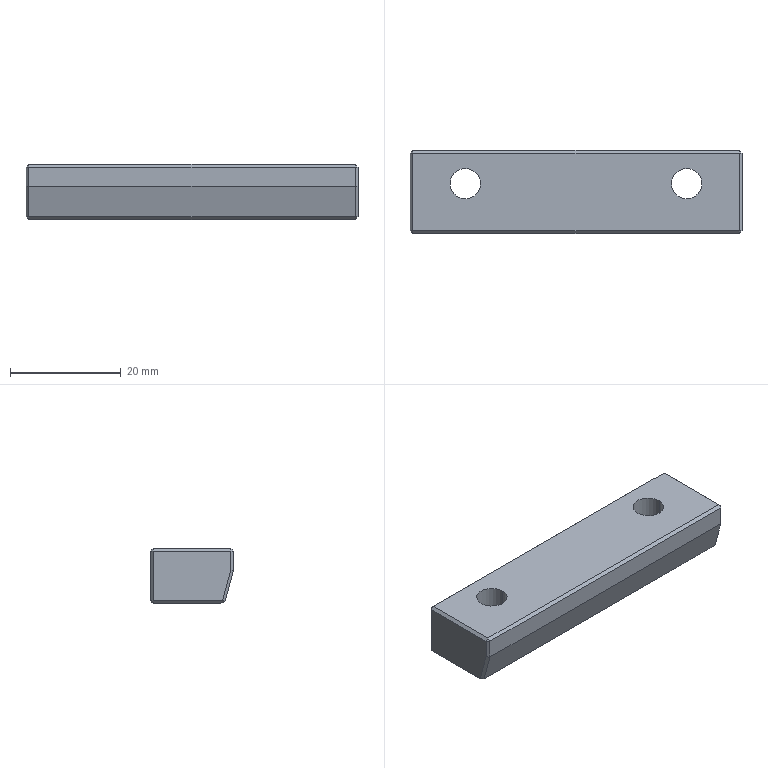Part | STEP file | KF-2212-010-049 | 1 solid | 39 faces | box 60 x 15 x 10 mm | volume 7567 mm3 | plane 31 | cylinder 8 | commonest cylinder face diameters 5.5 x4 10 x4
STEP:
#1=CARTESIAN_POINT('',(-119.63,635.5,-4.3));
#2=VERTEX_POINT('',#1);
#3=CARTESIAN_POINT('',(-129.63,635.5,-4.3));
#4=VERTEX_POINT('',#3);
#5=CARTESIAN_POINT('',(-124.63,635.5,-4.3));
#6=DIRECTION('',(0.,0.,-1.));
#7=DIRECTION('',(-1.,0.,0.));
#8=AXIS2_PLACEMENT_3D('',#5,#6,#7);
#9=CIRCLE('',#8,5.);
#10=EDGE_CURVE('',#2,#4,#9,.T.);
#11=ORIENTED_EDGE('',*,*,#10,.F.);
#12=CARTESIAN_POINT('',(-119.63,635.5,-10.));
#13=VERTEX_POINT('',#12);
#14=CARTESIAN_POINT('',(-119.63,635.5,-10.));
#15=DIRECTION('',(0.,0.,-1.));
#16=VECTOR('',#15,1000.);
#17=LINE('',#14,#16);
#18=EDGE_CURVE('',#2,#13,#17,.T.);
#19=ORIENTED_EDGE('',*,*,#18,.T.);
#20=CARTESIAN_POINT('',(-129.63,635.5,-10.));
#21=VERTEX_POINT('',#20);
#22=CARTESIAN_POINT('',(-124.63,635.5,-10.));
#23=DIRECTION('',(0.,0.,-1.));
#24=DIRECTION('',(-1.,0.,0.));
#25=AXIS2_PLACEMENT_3D('',#22,#23,#24);
#26=CIRCLE('',#25,5.);
#27=EDGE_CURVE('',#13,#21,#26,.T.);
#28=ORIENTED_EDGE('',*,*,#27,.T.);
#29=CARTESIAN_POINT('',(-129.63,635.5,-10.));
#30=DIRECTION('',(0.,0.,-1.));
#31=VECTOR('',#30,1000.);
#32=LINE('',#29,#31);
#33=EDGE_CURVE('',#4,#21,#32,.T.);
#34=ORIENTED_EDGE('',*,*,#33,.F.);
#35=EDGE_LOOP('',(#11,#19,#28,#34));
#36=FACE_OUTER_BOUND('',#35,.T.);
#37=CARTESIAN_POINT('',(-124.63,635.5,-10.));
#38=DIRECTION('',(0.,0.,-1.));
#39=DIRECTION('',(-1.,0.,0.));
#40=AXIS2_PLACEMENT_3D('',#37,#38,#39);
#41=CYLINDRICAL_SURFACE('',#40,5.);
#42=ADVANCED_FACE('',(#36),#41,.F.);
#43=CARTESIAN_POINT('',(-121.88,635.5,0.));
#44=VERTEX_POINT('',#43);
#45=CARTESIAN_POINT('',(-127.38,635.5,0.));
#46=VERTEX_POINT('',#45);
#47=CARTESIAN_POINT('',(-124.63,635.5,0.));
#48=DIRECTION('',(0.,0.,-1.));
#49=DIRECTION('',(-1.,0.,0.));
#50=AXIS2_PLACEMENT_3D('',#47,#48,#49);
#51=CIRCLE('',#50,2.75);
#52=EDGE_CURVE('',#44,#46,#51,.T.);
#53=ORIENTED_EDGE('',*,*,#52,.F.);
#54=CARTESIAN_POINT('',(-121.88,635.5,-4.3));
#55=VERTEX_POINT('',#54);
#56=CARTESIAN_POINT('',(-121.88,635.5,-10.));
#57=DIRECTION('',(0.,0.,-1.));
#58=VECTOR('',#57,1000.);
#59=LINE('',#56,#58);
#60=EDGE_CURVE('',#44,#55,#59,.T.);
#61=ORIENTED_EDGE('',*,*,#60,.T.);
#62=CARTESIAN_POINT('',(-127.38,635.5,-4.3));
#63=VERTEX_POINT('',#62);
#64=CARTESIAN_POINT('',(-124.63,635.5,-4.3));
#65=DIRECTION('',(0.,0.,-1.));
#66=DIRECTION('',(-1.,0.,0.));
#67=AXIS2_PLACEMENT_3D('',#64,#65,#66);
#68=CIRCLE('',#67,2.75);
#69=EDGE_CURVE('',#55,#63,#68,.T.);
#70=ORIENTED_EDGE('',*,*,#69,.T.);
#71=CARTESIAN_POINT('',(-127.38,635.5,-10.));
#72=DIRECTION('',(0.,0.,-1.));
#73=VECTOR('',#72,1000.);
#74=LINE('',#71,#73);
#75=EDGE_CURVE('',#46,#63,#74,.T.);
#76=ORIENTED_EDGE('',*,*,#75,.F.);
#77=EDGE_LOOP('',(#53,#61,#70,#76));
#78=FACE_OUTER_BOUND('',#77,.T.);
#79=CARTESIAN_POINT('',(-124.63,635.5,-10.));
#80=DIRECTION('',(0.,0.,-1.));
#81=DIRECTION('',(-1.,0.,0.));
#82=AXIS2_PLACEMENT_3D('',#79,#80,#81);
#83=CYLINDRICAL_SURFACE('',#82,2.75);
#84=ADVANCED_FACE('',(#78),#83,.F.);
#85=CARTESIAN_POINT('',(-159.63,635.5,-4.3));
#86=VERTEX_POINT('',#85);
#87=CARTESIAN_POINT('',(-169.63,635.5,-4.3));
#88=VERTEX_POINT('',#87);
#89=CARTESIAN_POINT('',(-164.63,635.5,-4.3));
#90=DIRECTION('',(0.,0.,-1.));
#91=DIRECTION('',(-1.,0.,0.));
#92=AXIS2_PLACEMENT_3D('',#89,#90,#91);
#93=CIRCLE('',#92,5.);
#94=EDGE_CURVE('',#86,#88,#93,.T.);
#95=ORIENTED_EDGE('',*,*,#94,.F.);
#96=CARTESIAN_POINT('',(-159.63,635.5,-10.));
#97=VERTEX_POINT('',#96);
#98=CARTESIAN_POINT('',(-159.63,635.5,-10.));
#99=DIRECTION('',(0.,0.,-1.));
#100=VECTOR('',#99,1000.);
#101=LINE('',#98,#100);
#102=EDGE_CURVE('',#86,#97,#101,.T.);
#103=ORIENTED_EDGE('',*,*,#102,.T.);
#104=CARTESIAN_POINT('',(-169.63,635.5,-10.));
#105=VERTEX_POINT('',#104);
#106=CARTESIAN_POINT('',(-164.63,635.5,-10.));
#107=DIRECTION('',(0.,0.,-1.));
#108=DIRECTION('',(-1.,0.,0.));
#109=AXIS2_PLACEMENT_3D('',#106,#107,#108);
#110=CIRCLE('',#109,5.);
#111=EDGE_CURVE('',#97,#105,#110,.T.);
#112=ORIENTED_EDGE('',*,*,#111,.T.);
#113=CARTESIAN_POINT('',(-169.63,635.5,-10.));
#114=DIRECTION('',(0.,0.,-1.));
#115=VECTOR('',#114,1000.);
#116=LINE('',#113,#115);
#117=EDGE_CURVE('',#88,#105,#116,.T.);
#118=ORIENTED_EDGE('',*,*,#117,.F.);
#119=EDGE_LOOP('',(#95,#103,#112,#118));
#120=FACE_OUTER_BOUND('',#119,.T.);
#121=CARTESIAN_POINT('',(-164.63,635.5,-10.));
#122=DIRECTION('',(0.,0.,-1.));
#123=DIRECTION('',(-1.,0.,0.));
#124=AXIS2_PLACEMENT_3D('',#121,#122,#123);
#125=CYLINDRICAL_SURFACE('',#124,5.);
#126=ADVANCED_FACE('',(#120),#125,.F.);
#127=CARTESIAN_POINT('',(-161.88,635.5,0.));
#128=VERTEX_POINT('',#127);
#129=CARTESIAN_POINT('',(-167.38,635.5,0.));
#130=VERTEX_POINT('',#129);
#131=CARTESIAN_POINT('',(-164.63,635.5,0.));
#132=DIRECTION('',(0.,0.,-1.));
#133=DIRECTION('',(-1.,0.,0.));
#134=AXIS2_PLACEMENT_3D('',#131,#132,#133);
#135=CIRCLE('',#134,2.75);
#136=EDGE_CURVE('',#128,#130,#135,.T.);
#137=ORIENTED_EDGE('',*,*,#136,.F.);
#138=CARTESIAN_POINT('',(-161.88,635.5,-4.3));
#139=VERTEX_POINT('',#138);
#140=CARTESIAN_POINT('',(-161.88,635.5,-10.));
#141=DIRECTION('',(0.,0.,-1.));
#142=VECTOR('',#141,1000.);
#143=LINE('',#140,#142);
#144=EDGE_CURVE('',#128,#139,#143,.T.);
#145=ORIENTED_EDGE('',*,*,#144,.T.);
#146=CARTESIAN_POINT('',(-167.38,635.5,-4.3));
#147=VERTEX_POINT('',#146);
#148=CARTESIAN_POINT('',(-164.63,635.5,-4.3));
#149=DIRECTION('',(0.,0.,-1.));
#150=DIRECTION('',(-1.,0.,0.));
#151=AXIS2_PLACEMENT_3D('',#148,#149,#150);
#152=CIRCLE('',#151,2.75);
#153=EDGE_CURVE('',#139,#147,#152,.T.);
#154=ORIENTED_EDGE('',*,*,#153,.T.);
#155=CARTESIAN_POINT('',(-167.38,635.5,-10.));
#156=DIRECTION('',(0.,0.,-1.));
#157=VECTOR('',#156,1000.);
#158=LINE('',#155,#157);
#159=EDGE_CURVE('',#130,#147,#158,.T.);
#160=ORIENTED_EDGE('',*,*,#159,.F.);
#161=EDGE_LOOP('',(#137,#145,#154,#160));
#162=FACE_OUTER_BOUND('',#161,.T.);
#163=CARTESIAN_POINT('',(-164.63,635.5,-10.));
#164=DIRECTION('',(0.,0.,-1.));
#165=DIRECTION('',(-1.,0.,0.));
#166=AXIS2_PLACEMENT_3D('',#163,#164,#165);
#167=CYLINDRICAL_SURFACE('',#166,2.75);
#168=ADVANCED_FACE('',(#162),#167,.F.);
#169=CARTESIAN_POINT('',(-174.63,627.,-0.5));
#170=VERTEX_POINT('',#169);
#171=CARTESIAN_POINT('',(-174.63,641.,-0.5));
#172=VERTEX_POINT('',#171);
#173=CARTESIAN_POINT('',(-174.63,641.5,-0.5));
#174=DIRECTION('',(0.,1.,0.));
#175=VECTOR('',#174,1000.);
#176=LINE('',#173,#175);
#177=EDGE_CURVE('',#170,#172,#176,.T.);
#178=ORIENTED_EDGE('',*,*,#177,.T.);
#179=CARTESIAN_POINT('',(-174.63,641.,-9.5));
#180=VERTEX_POINT('',#179);
#181=CARTESIAN_POINT('',(-174.63,641.,-10.));
#182=DIRECTION('',(0.,0.,-1.));
#183=VECTOR('',#182,1000.);
#184=LINE('',#181,#183);
#185=EDGE_CURVE('',#172,#180,#184,.T.);
#186=ORIENTED_EDGE('',*,*,#185,.T.);
#187=CARTESIAN_POINT('',(-174.63,628.492,-9.5));
#188=VERTEX_POINT('',#187);
#189=CARTESIAN_POINT('',(-174.63,626.5,-9.5));
#190=DIRECTION('',(0.,-1.,0.));
#191=VECTOR('',#190,1000.);
#192=LINE('',#189,#191);
#193=EDGE_CURVE('',#180,#188,#192,.T.);
#194=ORIENTED_EDGE('',*,*,#193,.T.);
#195=CARTESIAN_POINT('',(-174.63,627.,-3.934));
#196=VERTEX_POINT('',#195);
#197=CARTESIAN_POINT('',(-174.63,628.483,-9.469));
#198=DIRECTION('',(0.,-0.2588,0.9659));
#199=VECTOR('',#198,1000.);
#200=LINE('',#197,#199);
#201=EDGE_CURVE('',#188,#196,#200,.T.);
#202=ORIENTED_EDGE('',*,*,#201,.T.);
#203=CARTESIAN_POINT('',(-174.63,627.,-10.));
#204=DIRECTION('',(0.,0.,1.));
#205=VECTOR('',#204,1000.);
#206=LINE('',#203,#205);
#207=EDGE_CURVE('',#196,#170,#206,.T.);
#208=ORIENTED_EDGE('',*,*,#207,.T.);
#209=EDGE_LOOP('',(#178,#186,#194,#202,#208));
#210=FACE_OUTER_BOUND('',#209,.T.);
#211=CARTESIAN_POINT('',(-174.63,626.5,-10.));
#212=DIRECTION('',(-1.,0.,0.));
#213=DIRECTION('',(0.,0.,1.));
#214=AXIS2_PLACEMENT_3D('',#211,#212,#213);
#215=PLANE('',#214);
#216=ADVANCED_FACE('',(#210),#215,.T.);
#217=CARTESIAN_POINT('',(-115.13,641.5,-0.5));
#218=VERTEX_POINT('',#217);
#219=CARTESIAN_POINT('',(-115.13,641.5,-9.5));
#220=VERTEX_POINT('',#219);
#221=CARTESIAN_POINT('',(-115.13,641.5,-10.));
#222=DIRECTION('',(0.,0.,-1.));
#223=VECTOR('',#222,1000.);
#224=LINE('',#221,#223);
#225=EDGE_CURVE('',#218,#220,#224,.T.);
#226=ORIENTED_EDGE('',*,*,#225,.T.);
#227=CARTESIAN_POINT('',(-174.13,641.5,-9.5));
#228=VERTEX_POINT('',#227);
#229=CARTESIAN_POINT('',(-174.63,641.5,-9.5));
#230=DIRECTION('',(-1.,0.,0.));
#231=VECTOR('',#230,1000.);
#232=LINE('',#229,#231);
#233=EDGE_CURVE('',#220,#228,#232,.T.);
#234=ORIENTED_EDGE('',*,*,#233,.T.);
#235=CARTESIAN_POINT('',(-174.13,641.5,-0.5));
#236=VERTEX_POINT('',#235);
#237=CARTESIAN_POINT('',(-174.13,641.5,-10.));
#238=DIRECTION('',(0.,0.,1.));
#239=VECTOR('',#238,1000.);
#240=LINE('',#237,#239);
#241=EDGE_CURVE('',#228,#236,#240,.T.);
#242=ORIENTED_EDGE('',*,*,#241,.T.);
#243=CARTESIAN_POINT('',(-114.63,641.5,-0.5));
#244=DIRECTION('',(1.,0.,0.));
#245=VECTOR('',#244,1000.);
#246=LINE('',#243,#245);
#247=EDGE_CURVE('',#236,#218,#246,.T.);
#248=ORIENTED_EDGE('',*,*,#247,.T.);
#249=EDGE_LOOP('',(#226,#234,#242,#248));
#250=FACE_OUTER_BOUND('',#249,.T.);
#251=CARTESIAN_POINT('',(-174.63,641.5,-10.));
#252=DIRECTION('',(0.,1.,0.));
#253=DIRECTION('',(0.,0.,1.));
#254=AXIS2_PLACEMENT_3D('',#251,#252,#253);
#255=PLANE('',#254);
#256=ADVANCED_FACE('',(#250),#255,.T.);
#257=CARTESIAN_POINT('',(-114.63,627.,-3.934));
#258=VERTEX_POINT('',#257);
#259=CARTESIAN_POINT('',(-114.63,628.492,-9.5));
#260=VERTEX_POINT('',#259);
#261=CARTESIAN_POINT('',(-114.63,628.483,-9.469));
#262=DIRECTION('',(0.,0.2588,-0.9659));
#263=VECTOR('',#262,1000.);
#264=LINE('',#261,#263);
#265=EDGE_CURVE('',#258,#260,#264,.T.);
#266=ORIENTED_EDGE('',*,*,#265,.T.);
#267=CARTESIAN_POINT('',(-114.63,641.,-9.5));
#268=VERTEX_POINT('',#267);
#269=CARTESIAN_POINT('',(-114.63,626.5,-9.5));
#270=DIRECTION('',(0.,1.,0.));
#271=VECTOR('',#270,1000.);
#272=LINE('',#269,#271);
#273=EDGE_CURVE('',#260,#268,#272,.T.);
#274=ORIENTED_EDGE('',*,*,#273,.T.);
#275=CARTESIAN_POINT('',(-114.63,641.,-0.5));
#276=VERTEX_POINT('',#275);
#277=CARTESIAN_POINT('',(-114.63,641.,-10.));
#278=DIRECTION('',(0.,0.,1.));
#279=VECTOR('',#278,1000.);
#280=LINE('',#277,#279);
#281=EDGE_CURVE('',#268,#276,#280,.T.);
#282=ORIENTED_EDGE('',*,*,#281,.T.);
#283=CARTESIAN_POINT('',(-114.63,627.,-0.5));
#284=VERTEX_POINT('',#283);
#285=CARTESIAN_POINT('',(-114.63,626.5,-0.5));
#286=DIRECTION('',(0.,-1.,0.));
#287=VECTOR('',#286,1000.);
#288=LINE('',#285,#287);
#289=EDGE_CURVE('',#276,#284,#288,.T.);
#290=ORIENTED_EDGE('',*,*,#289,.T.);
#291=CARTESIAN_POINT('',(-114.63,627.,-10.));
#292=DIRECTION('',(0.,0.,-1.));
#293=VECTOR('',#292,1000.);
#294=LINE('',#291,#293);
#295=EDGE_CURVE('',#284,#258,#294,.T.);
#296=ORIENTED_EDGE('',*,*,#295,.T.);
#297=EDGE_LOOP('',(#266,#274,#282,#290,#296));
#298=FACE_OUTER_BOUND('',#297,.T.);
#299=CARTESIAN_POINT('',(-114.63,626.5,-10.));
#300=DIRECTION('',(1.,0.,0.));
#301=DIRECTION('',(0.,0.,-1.));
#302=AXIS2_PLACEMENT_3D('',#299,#300,#301);
#303=PLANE('',#302);
#304=ADVANCED_FACE('',(#298),#303,.T.);
#305=CARTESIAN_POINT('',(-174.13,626.5,-4.));
#306=VERTEX_POINT('',#305);
#307=CARTESIAN_POINT('',(-115.13,626.5,-4.));
#308=VERTEX_POINT('',#307);
#309=CARTESIAN_POINT('',(-174.63,626.5,-4.));
#310=DIRECTION('',(1.,0.,0.));
#311=VECTOR('',#310,1000.);
#312=LINE('',#309,#311);
#313=EDGE_CURVE('',#306,#308,#312,.T.);
#314=ORIENTED_EDGE('',*,*,#313,.T.);
#315=CARTESIAN_POINT('',(-115.13,626.5,-0.5));
#316=VERTEX_POINT('',#315);
#317=CARTESIAN_POINT('',(-115.13,626.5,-10.));
#318=DIRECTION('',(0.,0.,1.));
#319=VECTOR('',#318,1000.);
#320=LINE('',#317,#319);
#321=EDGE_CURVE('',#308,#316,#320,.T.);
#322=ORIENTED_EDGE('',*,*,#321,.T.);
#323=CARTESIAN_POINT('',(-174.13,626.5,-0.5));
#324=VERTEX_POINT('',#323);
#325=CARTESIAN_POINT('',(-174.63,626.5,-0.5));
#326=DIRECTION('',(-1.,0.,0.));
#327=VECTOR('',#326,1000.);
#328=LINE('',#325,#327);
#329=EDGE_CURVE('',#316,#324,#328,.T.);
#330=ORIENTED_EDGE('',*,*,#329,.T.);
#331=CARTESIAN_POINT('',(-174.13,626.5,-10.));
#332=DIRECTION('',(0.,0.,-1.));
#333=VECTOR('',#332,1000.);
#334=LINE('',#331,#333);
#335=EDGE_CURVE('',#324,#306,#334,.T.);
#336=ORIENTED_EDGE('',*,*,#335,.T.);
#337=EDGE_LOOP('',(#314,#322,#330,#336));
#338=FACE_OUTER_BOUND('',#337,.T.);
#339=CARTESIAN_POINT('',(-174.63,626.5,-10.));
#340=DIRECTION('',(0.,-1.,0.));
#341=DIRECTION('',(0.,0.,-1.));
#342=AXIS2_PLACEMENT_3D('',#339,#340,#341);
#343=PLANE('',#342);
#344=ADVANCED_FACE('',(#338),#343,.T.);
#345=CARTESIAN_POINT('',(-124.63,635.5,-10.));
#346=DIRECTION('',(0.,0.,-1.));
#347=DIRECTION('',(-1.,0.,0.));
#348=AXIS2_PLACEMENT_3D('',#345,#346,#347);
#349=CIRCLE('',#348,5.);
#350=EDGE_CURVE('',#21,#13,#349,.T.);
#351=ORIENTED_EDGE('',*,*,#350,.F.);
#352=ORIENTED_EDGE('',*,*,#27,.F.);
#353=EDGE_LOOP('',(#351,#352));
#354=FACE_BOUND('',#353,.T.);
#355=CARTESIAN_POINT('',(-164.63,635.5,-10.));
#356=DIRECTION('',(0.,0.,-1.));
#357=DIRECTION('',(-1.,0.,0.));
#358=AXIS2_PLACEMENT_3D('',#355,#356,#357);
#359=CIRCLE('',#358,5.);
#360=EDGE_CURVE('',#105,#97,#359,.T.);
#361=ORIENTED_EDGE('',*,*,#360,.F.);
#362=ORIENTED_EDGE('',*,*,#111,.F.);
#363=EDGE_LOOP('',(#361,#362));
#364=FACE_BOUND('',#363,.T.);
#365=CARTESIAN_POINT('',(-115.13,641.,-10.));
#366=VERTEX_POINT('',#365);
#367=CARTESIAN_POINT('',(-115.13,628.815,-10.));
#368=VERTEX_POINT('',#367);
#369=CARTESIAN_POINT('',(-115.13,0.,-10.));
#370=DIRECTION('',(0.,-1.,0.));
#371=VECTOR('',#370,1000.);
#372=LINE('',#369,#371);
#373=EDGE_CURVE('',#366,#368,#372,.T.);
#374=ORIENTED_EDGE('',*,*,#373,.T.);
#375=CARTESIAN_POINT('',(-174.13,628.815,-10.));
#376=VERTEX_POINT('',#375);
#377=CARTESIAN_POINT('',(0.,628.815,-10.));
#378=DIRECTION('',(-1.,0.,0.));
#379=VECTOR('',#378,1000.);
#380=LINE('',#377,#379);
#381=EDGE_CURVE('',#368,#376,#380,.T.);
#382=ORIENTED_EDGE('',*,*,#381,.T.);
#383=CARTESIAN_POINT('',(-174.13,641.,-10.));
#384=VERTEX_POINT('',#383);
#385=CARTESIAN_POINT('',(-174.13,0.,-10.));
#386=DIRECTION('',(0.,1.,0.));
#387=VECTOR('',#386,1000.);
#388=LINE('',#385,#387);
#389=EDGE_CURVE('',#376,#384,#388,.T.);
#390=ORIENTED_EDGE('',*,*,#389,.T.);
#391=CARTESIAN_POINT('',(0.,641.,-10.));
#392=DIRECTION('',(1.,0.,0.));
#393=VECTOR('',#392,1000.);
#394=LINE('',#391,#393);
#395=EDGE_CURVE('',#384,#366,#394,.T.);
#396=ORIENTED_EDGE('',*,*,#395,.T.);
#397=EDGE_LOOP('',(#374,#382,#390,#396));
#398=FACE_OUTER_BOUND('',#397,.T.);
#399=CARTESIAN_POINT('',(0.,0.,-10.));
#400=DIRECTION('',(0.,0.,-1.));
#401=DIRECTION('',(-1.,0.,0.));
#402=AXIS2_PLACEMENT_3D('',#399,#400,#401);
#403=PLANE('',#402);
#404=ADVANCED_FACE('',(#354,#364,#398),#403,.T.);
#405=CARTESIAN_POINT('',(-124.63,635.5,0.));
#406=DIRECTION('',(0.,0.,-1.));
#407=DIRECTION('',(-1.,0.,0.));
#408=AXIS2_PLACEMENT_3D('',#405,#406,#407);
#409=CIRCLE('',#408,2.75);
#410=EDGE_CURVE('',#46,#44,#409,.T.);
#411=ORIENTED_EDGE('',*,*,#410,.T.);
#412=ORIENTED_EDGE('',*,*,#52,.T.);
#413=EDGE_LOOP('',(#411,#412));
#414=FACE_BOUND('',#413,.T.);
#415=CARTESIAN_POINT('',(-164.63,635.5,0.));
#416=DIRECTION('',(0.,0.,-1.));
#417=DIRECTION('',(-1.,0.,0.));
#418=AXIS2_PLACEMENT_3D('',#415,#416,#417);
#419=CIRCLE('',#418,2.75);
#420=EDGE_CURVE('',#130,#128,#419,.T.);
#421=ORIENTED_EDGE('',*,*,#420,.T.);
#422=ORIENTED_EDGE('',*,*,#136,.T.);
#423=EDGE_LOOP('',(#421,#422));
#424=FACE_BOUND('',#423,.T.);
#425=CARTESIAN_POINT('',(-115.13,627.,0.));
#426=VERTEX_POINT('',#425);
#427=CARTESIAN_POINT('',(-115.13,641.,0.));
#428=VERTEX_POINT('',#427);
#429=CARTESIAN_POINT('',(-115.13,641.5,0.));
#430=DIRECTION('',(0.,1.,0.));
#431=VECTOR('',#430,1000.);
#432=LINE('',#429,#431);
#433=EDGE_CURVE('',#426,#428,#432,.T.);
#434=ORIENTED_EDGE('',*,*,#433,.T.);
#435=CARTESIAN_POINT('',(-174.13,641.,0.));
#436=VERTEX_POINT('',#435);
#437=CARTESIAN_POINT('',(-174.63,641.,0.));
#438=DIRECTION('',(-1.,0.,0.));
#439=VECTOR('',#438,1000.);
#440=LINE('',#437,#439);
#441=EDGE_CURVE('',#428,#436,#440,.T.);
#442=ORIENTED_EDGE('',*,*,#441,.T.);
#443=CARTESIAN_POINT('',(-174.13,627.,0.));
#444=VERTEX_POINT('',#443);
#445=CARTESIAN_POINT('',(-174.13,626.5,0.));
#446=DIRECTION('',(0.,-1.,0.));
#447=VECTOR('',#446,1000.);
#448=LINE('',#445,#447);
#449=EDGE_CURVE('',#436,#444,#448,.T.);
#450=ORIENTED_EDGE('',*,*,#449,.T.);
#451=CARTESIAN_POINT('',(-114.63,627.,0.));
#452=DIRECTION('',(1.,0.,0.));
#453=VECTOR('',#452,1000.);
#454=LINE('',#451,#453);
#455=EDGE_CURVE('',#444,#426,#454,.T.);
#456=ORIENTED_EDGE('',*,*,#455,.T.);
#457=EDGE_LOOP('',(#434,#442,#450,#456));
#458=FACE_OUTER_BOUND('',#457,.T.);
#459=CARTESIAN_POINT('',(0.,0.,0.));
#460=DIRECTION('',(0.,0.,-1.));
#461=DIRECTION('',(-1.,0.,0.));
#462=AXIS2_PLACEMENT_3D('',#459,#460,#461);
#463=PLANE('',#462);
#464=ADVANCED_FACE('',(#414,#424,#458),#463,.F.);
#465=CARTESIAN_POINT('',(-174.13,627.978,-9.517));
#466=VERTEX_POINT('',#465);
#467=CARTESIAN_POINT('',(-115.13,627.978,-9.517));
#468=VERTEX_POINT('',#467);
#469=CARTESIAN_POINT('',(-174.63,627.978,-9.517));
#470=DIRECTION('',(1.,0.,0.));
#471=VECTOR('',#470,1000.);
#472=LINE('',#469,#471);
#473=EDGE_CURVE('',#466,#468,#472,.T.);
#474=ORIENTED_EDGE('',*,*,#473,.T.);
#475=CARTESIAN_POINT('',(-115.13,626.5,-4.));
#476=DIRECTION('',(0.,-0.2588,0.9659));
#477=VECTOR('',#476,1000.);
#478=LINE('',#475,#477);
#479=EDGE_CURVE('',#468,#308,#478,.T.);
#480=ORIENTED_EDGE('',*,*,#479,.T.);
#481=ORIENTED_EDGE('',*,*,#313,.F.);
#482=CARTESIAN_POINT('',(-174.13,626.5,-4.));
#483=DIRECTION('',(0.,0.2588,-0.9659));
#484=VECTOR('',#483,1000.);
#485=LINE('',#482,#484);
#486=EDGE_CURVE('',#306,#466,#485,.T.);
#487=ORIENTED_EDGE('',*,*,#486,.T.);
#488=EDGE_LOOP('',(#474,#480,#481,#487));
#489=FACE_OUTER_BOUND('',#488,.T.);
#490=CARTESIAN_POINT('',(-174.63,626.5,-4.));
#491=DIRECTION('',(0.,0.9659,0.2588));
#492=DIRECTION('',(1.,0.,0.));
#493=AXIS2_PLACEMENT_3D('',#490,#491,#492);
#494=PLANE('',#493);
#495=ADVANCED_FACE('',(#489),#494,.F.);
#496=CARTESIAN_POINT('',(-174.13,641.5,-0.5));
#497=DIRECTION('',(0.,0.7071,-0.7071));
#498=VECTOR('',#497,1000.);
#499=LINE('',#496,#498);
#500=EDGE_CURVE('',#436,#236,#499,.T.);
#501=ORIENTED_EDGE('',*,*,#500,.F.);
#502=ORIENTED_EDGE('',*,*,#441,.F.);
#503=CARTESIAN_POINT('',(-115.13,641.25,-0.25));
#504=DIRECTION('',(0.,-0.7071,0.7071));
#505=VECTOR('',#504,1000.);
#506=LINE('',#503,#505);
#507=EDGE_CURVE('',#218,#428,#506,.T.);
#508=ORIENTED_EDGE('',*,*,#507,.F.);
#509=ORIENTED_EDGE('',*,*,#247,.F.);
#510=EDGE_LOOP('',(#501,#502,#508,#509));
#511=FACE_OUTER_BOUND('',#510,.T.);
#512=CARTESIAN_POINT('',(0.,641.,0.));
#513=DIRECTION('',(0.,0.7071,0.7071));
#514=DIRECTION('',(1.,0.,0.));
#515=AXIS2_PLACEMENT_3D('',#512,#513,#514);
#516=PLANE('',#515);
#517=ADVANCED_FACE('',(#511),#516,.T.);
#518=CARTESIAN_POINT('',(-114.63,641.,-0.5));
#519=DIRECTION('',(0.7071,0.,-0.7071));
#520=VECTOR('',#519,1000.);
#521=LINE('',#518,#520);
#522=EDGE_CURVE('',#428,#276,#521,.T.);
#523=ORIENTED_EDGE('',*,*,#522,.F.);
#524=ORIENTED_EDGE('',*,*,#433,.F.);
#525=CARTESIAN_POINT('',(-114.88,627.,-0.25));
#526=DIRECTION('',(-0.7071,0.,0.7071));
#527=VECTOR('',#526,1000.);
#528=LINE('',#525,#527);
#529=EDGE_CURVE('',#284,#426,#528,.T.);
#530=ORIENTED_EDGE('',*,*,#529,.F.);
#531=ORIENTED_EDGE('',*,*,#289,.F.);
#532=EDGE_LOOP('',(#523,#524,#530,#531));
#533=FACE_OUTER_BOUND('',#532,.T.);
#534=CARTESIAN_POINT('',(-115.13,0.,0.));
#535=DIRECTION('',(0.7071,0.,0.7071));
#536=DIRECTION('',(0.,-1.,0.));
#537=AXIS2_PLACEMENT_3D('',#534,#535,#536);
#538=PLANE('',#537);
#539=ADVANCED_FACE('',(#533),#538,.T.);
#540=ORIENTED_EDGE('',*,*,#507,.T.);
#541=ORIENTED_EDGE('',*,*,#522,.T.);
#542=CARTESIAN_POINT('',(-114.63,641.,-0.5));
#543=DIRECTION('',(0.7071,-0.7071,0.));
#544=VECTOR('',#543,1000.);
#545=LINE('',#542,#544);
#546=EDGE_CURVE('',#218,#276,#545,.T.);
#547=ORIENTED_EDGE('',*,*,#546,.F.);
#548=EDGE_LOOP('',(#540,#541,#547));
#549=FACE_OUTER_BOUND('',#548,.T.);
#550=CARTESIAN_POINT('',(-114.63,641.,-0.5));
#551=DIRECTION('',(0.5774,0.5774,0.5774));
#552=DIRECTION('',(-0.7071,0.7071,0.));
#553=AXIS2_PLACEMENT_3D('',#550,#551,#552);
#554=PLANE('',#553);
#555=ADVANCED_FACE('',(#549),#554,.T.);
#556=CARTESIAN_POINT('',(-174.13,641.5,-0.5));
#557=DIRECTION('',(0.7071,0.7071,0.));
#558=VECTOR('',#557,1000.);
#559=LINE('',#556,#558);
#560=EDGE_CURVE('',#172,#236,#559,.T.);
#561=ORIENTED_EDGE('',*,*,#560,.F.);
#562=CARTESIAN_POINT('',(-174.38,641.,-0.25));
#563=DIRECTION('',(-0.7071,0.,-0.7071));
#564=VECTOR('',#563,1000.);
#565=LINE('',#562,#564);
#566=EDGE_CURVE('',#436,#172,#565,.T.);
#567=ORIENTED_EDGE('',*,*,#566,.F.);
#568=ORIENTED_EDGE('',*,*,#500,.T.);
#569=EDGE_LOOP('',(#561,#567,#568));
#570=FACE_OUTER_BOUND('',#569,.T.);
#571=CARTESIAN_POINT('',(-174.13,641.5,-0.5));
#572=DIRECTION('',(-0.5774,0.5774,0.5774));
#573=DIRECTION('',(-0.7071,-0.7071,0.));
#574=AXIS2_PLACEMENT_3D('',#571,#572,#573);
#575=PLANE('',#574);
#576=ADVANCED_FACE('',(#570),#575,.T.);
#577=ORIENTED_EDGE('',*,*,#566,.T.);
#578=ORIENTED_EDGE('',*,*,#177,.F.);
#579=CARTESIAN_POINT('',(-174.63,627.,-0.5));
#580=DIRECTION('',(-0.7071,0.,-0.7071));
#581=VECTOR('',#580,1000.);
#582=LINE('',#579,#581);
#583=EDGE_CURVE('',#444,#170,#582,.T.);
#584=ORIENTED_EDGE('',*,*,#583,.F.);
#585=ORIENTED_EDGE('',*,*,#449,.F.);
#586=EDGE_LOOP('',(#577,#578,#584,#585));
#587=FACE_OUTER_BOUND('',#586,.T.);
#588=CARTESIAN_POINT('',(-174.13,0.,0.));
#589=DIRECTION('',(-0.7071,0.,0.7071));
#590=DIRECTION('',(0.,1.,0.));
#591=AXIS2_PLACEMENT_3D('',#588,#589,#590);
#592=PLANE('',#591);
#593=ADVANCED_FACE('',(#587),#592,.T.);
#594=CARTESIAN_POINT('',(-115.13,626.5,-0.5));
#595=DIRECTION('',(0.,-0.7071,-0.7071));
#596=VECTOR('',#595,1000.);
#597=LINE('',#594,#596);
#598=EDGE_CURVE('',#426,#316,#597,.T.);
#599=ORIENTED_EDGE('',*,*,#598,.F.);
#600=ORIENTED_EDGE('',*,*,#455,.F.);
#601=CARTESIAN_POINT('',(-174.13,626.75,-0.25));
#602=DIRECTION('',(0.,0.7071,0.7071));
#603=VECTOR('',#602,1000.);
#604=LINE('',#601,#603);
#605=EDGE_CURVE('',#324,#444,#604,.T.);
#606=ORIENTED_EDGE('',*,*,#605,.F.);
#607=ORIENTED_EDGE('',*,*,#329,.F.);
#608=EDGE_LOOP('',(#599,#600,#606,#607));
#609=FACE_OUTER_BOUND('',#608,.T.);
#610=CARTESIAN_POINT('',(0.,627.,0.));
#611=DIRECTION('',(0.,-0.7071,0.7071));
#612=DIRECTION('',(-1.,0.,0.));
#613=AXIS2_PLACEMENT_3D('',#610,#611,#612);
#614=PLANE('',#613);
#615=ADVANCED_FACE('',(#609),#614,.T.);
#616=ORIENTED_EDGE('',*,*,#529,.T.);
#617=ORIENTED_EDGE('',*,*,#598,.T.);
#618=CARTESIAN_POINT('',(-115.13,626.5,-0.5));
#619=DIRECTION('',(-0.7071,-0.7071,0.));
#620=VECTOR('',#619,1000.);
#621=LINE('',#618,#620);
#622=EDGE_CURVE('',#284,#316,#621,.T.);
#623=ORIENTED_EDGE('',*,*,#622,.F.);
#624=EDGE_LOOP('',(#616,#617,#623));
#625=FACE_OUTER_BOUND('',#624,.T.);
#626=CARTESIAN_POINT('',(-115.13,626.5,-0.5));
#627=DIRECTION('',(0.5774,-0.5774,0.5774));
#628=DIRECTION('',(0.7071,0.,-0.7071));
#629=AXIS2_PLACEMENT_3D('',#626,#627,#628);
#630=PLANE('',#629);
#631=ADVANCED_FACE('',(#625),#630,.T.);
#632=ORIENTED_EDGE('',*,*,#546,.T.);
#633=ORIENTED_EDGE('',*,*,#281,.F.);
#634=CARTESIAN_POINT('',(-115.13,641.5,-9.5));
#635=DIRECTION('',(0.7071,-0.7071,0.));
#636=VECTOR('',#635,1000.);
#637=LINE('',#634,#636);
#638=EDGE_CURVE('',#220,#268,#637,.T.);
#639=ORIENTED_EDGE('',*,*,#638,.F.);
#640=ORIENTED_EDGE('',*,*,#225,.F.);
#641=EDGE_LOOP('',(#632,#633,#639,#640));
#642=FACE_OUTER_BOUND('',#641,.T.);
#643=CARTESIAN_POINT('',(-114.63,641.,-10.));
#644=DIRECTION('',(-0.7071,-0.7071,0.));
#645=DIRECTION('',(0.,0.,1.));
#646=AXIS2_PLACEMENT_3D('',#643,#644,#645);
#647=PLANE('',#646);
#648=ADVANCED_FACE('',(#642),#647,.F.);
#649=CARTESIAN_POINT('',(-174.13,641.25,-9.75));
#650=DIRECTION('',(0.,-0.7071,-0.7071));
#651=VECTOR('',#650,1000.);
#652=LINE('',#649,#651);
#653=EDGE_CURVE('',#228,#384,#652,.T.);
#654=ORIENTED_EDGE('',*,*,#653,.F.);
#655=ORIENTED_EDGE('',*,*,#233,.F.);
#656=CARTESIAN_POINT('',(-115.13,641.5,-9.5));
#657=DIRECTION('',(0.,0.7071,0.7071));
#658=VECTOR('',#657,1000.);
#659=LINE('',#656,#658);
#660=EDGE_CURVE('',#366,#220,#659,.T.);
#661=ORIENTED_EDGE('',*,*,#660,.F.);
#662=ORIENTED_EDGE('',*,*,#395,.F.);
#663=EDGE_LOOP('',(#654,#655,#661,#662));
#664=FACE_OUTER_BOUND('',#663,.T.);
#665=CARTESIAN_POINT('',(-174.63,641.5,-9.5));
#666=DIRECTION('',(0.,-0.7071,0.7071));
#667=DIRECTION('',(-1.,0.,0.));
#668=AXIS2_PLACEMENT_3D('',#665,#666,#667);
#669=PLANE('',#668);
#670=ADVANCED_FACE('',(#664),#669,.F.);
#671=ORIENTED_EDGE('',*,*,#560,.T.);
#672=ORIENTED_EDGE('',*,*,#241,.F.);
#673=CARTESIAN_POINT('',(-174.63,641.,-9.5));
#674=DIRECTION('',(0.7071,0.7071,0.));
#675=VECTOR('',#674,1000.);
#676=LINE('',#673,#675);
#677=EDGE_CURVE('',#180,#228,#676,.T.);
#678=ORIENTED_EDGE('',*,*,#677,.F.);
#679=ORIENTED_EDGE('',*,*,#185,.F.);
#680=EDGE_LOOP('',(#671,#672,#678,#679));
#681=FACE_OUTER_BOUND('',#680,.T.);
#682=CARTESIAN_POINT('',(-174.13,641.5,-10.));
#683=DIRECTION('',(0.7071,-0.7071,0.));
#684=DIRECTION('',(0.,0.,1.));
#685=AXIS2_PLACEMENT_3D('',#682,#683,#684);
#686=PLANE('',#685);
#687=ADVANCED_FACE('',(#681),#686,.F.);
#688=ORIENTED_EDGE('',*,*,#605,.T.);
#689=ORIENTED_EDGE('',*,*,#583,.T.);
#690=CARTESIAN_POINT('',(-174.63,627.,-0.5));
#691=DIRECTION('',(-0.7071,0.7071,0.));
#692=VECTOR('',#691,1000.);
#693=LINE('',#690,#692);
#694=EDGE_CURVE('',#324,#170,#693,.T.);
#695=ORIENTED_EDGE('',*,*,#694,.F.);
#696=EDGE_LOOP('',(#688,#689,#695));
#697=FACE_OUTER_BOUND('',#696,.T.);
#698=CARTESIAN_POINT('',(-174.63,627.,-0.5));
#699=DIRECTION('',(-0.5774,-0.5774,0.5774));
#700=DIRECTION('',(0.7071,0.,0.7071));
#701=AXIS2_PLACEMENT_3D('',#698,#699,#700);
#702=PLANE('',#701);
#703=ADVANCED_FACE('',(#697),#702,.T.);
#704=ORIENTED_EDGE('',*,*,#622,.T.);
#705=ORIENTED_EDGE('',*,*,#321,.F.);
#706=CARTESIAN_POINT('',(-115.522,626.109,-4.052));
#707=DIRECTION('',(-0.7041,-0.7041,-0.09269));
#708=VECTOR('',#707,1000.);
#709=LINE('',#706,#708);
#710=EDGE_CURVE('',#258,#308,#709,.T.);
#711=ORIENTED_EDGE('',*,*,#710,.F.);
#712=ORIENTED_EDGE('',*,*,#295,.F.);
#713=EDGE_LOOP('',(#704,#705,#711,#712));
#714=FACE_OUTER_BOUND('',#713,.T.);
#715=CARTESIAN_POINT('',(-115.13,626.5,-10.));
#716=DIRECTION('',(-0.7071,0.7071,0.));
#717=DIRECTION('',(0.,0.,1.));
#718=AXIS2_PLACEMENT_3D('',#715,#716,#717);
#719=PLANE('',#718);
#720=ADVANCED_FACE('',(#714),#719,.F.);
#721=ORIENTED_EDGE('',*,*,#660,.T.);
#722=ORIENTED_EDGE('',*,*,#638,.T.);
#723=CARTESIAN_POINT('',(-114.88,641.,-9.75));
#724=DIRECTION('',(0.7071,0.,0.7071));
#725=VECTOR('',#724,1000.);
#726=LINE('',#723,#725);
#727=EDGE_CURVE('',#366,#268,#726,.T.);
#728=ORIENTED_EDGE('',*,*,#727,.F.);
#729=EDGE_LOOP('',(#721,#722,#728));
#730=FACE_OUTER_BOUND('',#729,.T.);
#731=CARTESIAN_POINT('',(-115.13,641.5,-9.5));
#732=DIRECTION('',(0.5774,0.5774,-0.5774));
#733=DIRECTION('',(0.,0.7071,0.7071));
#734=AXIS2_PLACEMENT_3D('',#731,#732,#733);
#735=PLANE('',#734);
#736=ADVANCED_FACE('',(#730),#735,.T.);
#737=ORIENTED_EDGE('',*,*,#677,.T.);
#738=ORIENTED_EDGE('',*,*,#653,.T.);
#739=CARTESIAN_POINT('',(-174.63,641.,-9.5));
#740=DIRECTION('',(0.7071,0.,-0.7071));
#741=VECTOR('',#740,1000.);
#742=LINE('',#739,#741);
#743=EDGE_CURVE('',#180,#384,#742,.T.);
#744=ORIENTED_EDGE('',*,*,#743,.F.);
#745=EDGE_LOOP('',(#737,#738,#744));
#746=FACE_OUTER_BOUND('',#745,.T.);
#747=CARTESIAN_POINT('',(-174.63,641.,-9.5));
#748=DIRECTION('',(-0.5774,0.5774,-0.5774));
#749=DIRECTION('',(-0.7071,0.,0.7071));
#750=AXIS2_PLACEMENT_3D('',#747,#748,#749);
#751=PLANE('',#750);
#752=ADVANCED_FACE('',(#746),#751,.T.);
#753=ORIENTED_EDGE('',*,*,#694,.T.);
#754=ORIENTED_EDGE('',*,*,#207,.F.);
#755=CARTESIAN_POINT('',(-174.234,626.604,-3.986));
#756=DIRECTION('',(-0.7041,0.7041,0.09269));
#757=VECTOR('',#756,1000.);
#758=LINE('',#755,#757);
#759=EDGE_CURVE('',#306,#196,#758,.T.);
#760=ORIENTED_EDGE('',*,*,#759,.F.);
#761=ORIENTED_EDGE('',*,*,#335,.F.);
#762=EDGE_LOOP('',(#753,#754,#760,#761));
#763=FACE_OUTER_BOUND('',#762,.T.);
#764=CARTESIAN_POINT('',(-174.63,627.,-10.));
#765=DIRECTION('',(0.7071,0.7071,0.));
#766=DIRECTION('',(0.,0.,1.));
#767=AXIS2_PLACEMENT_3D('',#764,#765,#766);
#768=PLANE('',#767);
#769=ADVANCED_FACE('',(#763),#768,.F.);
#770=ORIENTED_EDGE('',*,*,#710,.T.);
#771=ORIENTED_EDGE('',*,*,#479,.F.);
#772=CARTESIAN_POINT('',(-115.13,627.978,-9.517));
#773=DIRECTION('',(-0.6977,-0.716,-0.02377));
#774=VECTOR('',#773,1000.);
#775=LINE('',#772,#774);
#776=EDGE_CURVE('',#260,#468,#775,.T.);
#777=ORIENTED_EDGE('',*,*,#776,.F.);
#778=ORIENTED_EDGE('',*,*,#265,.F.);
#779=EDGE_LOOP('',(#770,#771,#777,#778));
#780=FACE_OUTER_BOUND('',#779,.T.);
#781=CARTESIAN_POINT('',(-114.63,628.483,-9.469));
#782=DIRECTION('',(0.7071,-0.683,-0.183));
#783=DIRECTION('',(0.,-0.2588,0.9659));
#784=AXIS2_PLACEMENT_3D('',#781,#782,#783);
#785=PLANE('',#784);
#786=ADVANCED_FACE('',(#780),#785,.T.);
#787=ORIENTED_EDGE('',*,*,#727,.T.);
#788=ORIENTED_EDGE('',*,*,#273,.F.);
#789=CARTESIAN_POINT('',(-114.707,628.541,-9.577));
#790=DIRECTION('',(0.643,-0.416,0.643));
#791=VECTOR('',#790,1000.);
#792=LINE('',#789,#791);
#793=EDGE_CURVE('',#368,#260,#792,.T.);
#794=ORIENTED_EDGE('',*,*,#793,.F.);
#795=ORIENTED_EDGE('',*,*,#373,.F.);
#796=EDGE_LOOP('',(#787,#788,#794,#795));
#797=FACE_OUTER_BOUND('',#796,.T.);
#798=CARTESIAN_POINT('',(-114.63,626.5,-9.5));
#799=DIRECTION('',(-0.7071,0.,0.7071));
#800=DIRECTION('',(0.,1.,0.));
#801=AXIS2_PLACEMENT_3D('',#798,#799,#800);
#802=PLANE('',#801);
#803=ADVANCED_FACE('',(#797),#802,.F.);
#804=ORIENTED_EDGE('',*,*,#743,.T.);
#805=ORIENTED_EDGE('',*,*,#389,.F.);
#806=CARTESIAN_POINT('',(-174.13,628.815,-10.));
#807=DIRECTION('',(0.643,0.416,-0.643));
#808=VECTOR('',#807,1000.);
#809=LINE('',#806,#808);
#810=EDGE_CURVE('',#188,#376,#809,.T.);
#811=ORIENTED_EDGE('',*,*,#810,.F.);
#812=ORIENTED_EDGE('',*,*,#193,.F.);
#813=EDGE_LOOP('',(#804,#805,#811,#812));
#814=FACE_OUTER_BOUND('',#813,.T.);
#815=CARTESIAN_POINT('',(-174.63,626.5,-9.5));
#816=DIRECTION('',(0.7071,0.,0.7071));
#817=DIRECTION('',(0.,-1.,0.));
#818=AXIS2_PLACEMENT_3D('',#815,#816,#817);
#819=PLANE('',#818);
#820=ADVANCED_FACE('',(#814),#819,.F.);
#821=ORIENTED_EDGE('',*,*,#759,.T.);
#822=ORIENTED_EDGE('',*,*,#201,.F.);
#823=CARTESIAN_POINT('',(-174.54,628.399,-9.503));
#824=DIRECTION('',(-0.6977,0.716,0.02377));
#825=VECTOR('',#824,1000.);
#826=LINE('',#823,#825);
#827=EDGE_CURVE('',#466,#188,#826,.T.);
#828=ORIENTED_EDGE('',*,*,#827,.F.);
#829=ORIENTED_EDGE('',*,*,#486,.F.);
#830=EDGE_LOOP('',(#821,#822,#828,#829));
#831=FACE_OUTER_BOUND('',#830,.T.);
#832=CARTESIAN_POINT('',(-174.63,628.483,-9.469));
#833=DIRECTION('',(-0.7071,-0.683,-0.183));
#834=DIRECTION('',(0.,0.2588,-0.9659));
#835=AXIS2_PLACEMENT_3D('',#832,#833,#834);
#836=PLANE('',#835);
#837=ADVANCED_FACE('',(#831),#836,.T.);
#838=ORIENTED_EDGE('',*,*,#793,.T.);
#839=ORIENTED_EDGE('',*,*,#776,.T.);
#840=CARTESIAN_POINT('',(-115.13,627.978,-9.517));
#841=DIRECTION('',(0.,-0.866,0.5));
#842=VECTOR('',#841,1000.);
#843=LINE('',#840,#842);
#844=EDGE_CURVE('',#368,#468,#843,.T.);
#845=ORIENTED_EDGE('',*,*,#844,.F.);
#846=EDGE_LOOP('',(#838,#839,#845));
#847=FACE_OUTER_BOUND('',#846,.T.);
#848=CARTESIAN_POINT('',(-115.13,627.978,-9.517));
#849=DIRECTION('',(0.4769,-0.4395,-0.7612));
#850=DIRECTION('',(-0.8474,0.,-0.5309));
#851=AXIS2_PLACEMENT_3D('',#848,#849,#850);
#852=PLANE('',#851);
#853=ADVANCED_FACE('',(#847),#852,.T.);
#854=ORIENTED_EDGE('',*,*,#827,.T.);
#855=ORIENTED_EDGE('',*,*,#810,.T.);
#856=CARTESIAN_POINT('',(-174.13,628.815,-10.));
#857=DIRECTION('',(0.,0.866,-0.5));
#858=VECTOR('',#857,1000.);
#859=LINE('',#856,#858);
#860=EDGE_CURVE('',#466,#376,#859,.T.);
#861=ORIENTED_EDGE('',*,*,#860,.F.);
#862=EDGE_LOOP('',(#854,#855,#861));
#863=FACE_OUTER_BOUND('',#862,.T.);
#864=CARTESIAN_POINT('',(-174.13,628.815,-10.));
#865=DIRECTION('',(-0.4769,-0.4395,-0.7612));
#866=DIRECTION('',(-0.8474,0.,0.5309));
#867=AXIS2_PLACEMENT_3D('',#864,#865,#866);
#868=PLANE('',#867);
#869=ADVANCED_FACE('',(#863),#868,.T.);
#870=ORIENTED_EDGE('',*,*,#844,.T.);
#871=ORIENTED_EDGE('',*,*,#473,.F.);
#872=ORIENTED_EDGE('',*,*,#860,.T.);
#873=ORIENTED_EDGE('',*,*,#381,.F.);
#874=EDGE_LOOP('',(#870,#871,#872,#873));
#875=FACE_OUTER_BOUND('',#874,.T.);
#876=CARTESIAN_POINT('',(0.,628.815,-10.));
#877=DIRECTION('',(0.,-0.5,-0.866));
#878=DIRECTION('',(1.,0.,0.));
#879=AXIS2_PLACEMENT_3D('',#876,#877,#878);
#880=PLANE('',#879);
#881=ADVANCED_FACE('',(#875),#880,.T.);
#882=ORIENTED_EDGE('',*,*,#144,.F.);
#883=ORIENTED_EDGE('',*,*,#420,.F.);
#884=ORIENTED_EDGE('',*,*,#159,.T.);
#885=CARTESIAN_POINT('',(-164.63,635.5,-4.3));
#886=DIRECTION('',(0.,0.,-1.));
#887=DIRECTION('',(-1.,0.,0.));
#888=AXIS2_PLACEMENT_3D('',#885,#886,#887);
#889=CIRCLE('',#888,2.75);
#890=EDGE_CURVE('',#147,#139,#889,.T.);
#891=ORIENTED_EDGE('',*,*,#890,.T.);
#892=EDGE_LOOP('',(#882,#883,#884,#891));
#893=FACE_OUTER_BOUND('',#892,.T.);
#894=CARTESIAN_POINT('',(-164.63,635.5,-10.));
#895=DIRECTION('',(0.,0.,-1.));
#896=DIRECTION('',(-1.,0.,0.));
#897=AXIS2_PLACEMENT_3D('',#894,#895,#896);
#898=CYLINDRICAL_SURFACE('',#897,2.75);
#899=ADVANCED_FACE('',(#893),#898,.F.);
#900=ORIENTED_EDGE('',*,*,#890,.F.);
#901=ORIENTED_EDGE('',*,*,#153,.F.);
#902=EDGE_LOOP('',(#900,#901));
#903=FACE_BOUND('',#902,.T.);
#904=CARTESIAN_POINT('',(-164.63,635.5,-4.3));
#905=DIRECTION('',(0.,0.,-1.));
#906=DIRECTION('',(-1.,0.,0.));
#907=AXIS2_PLACEMENT_3D('',#904,#905,#906);
#908=CIRCLE('',#907,5.);
#909=EDGE_CURVE('',#88,#86,#908,.T.);
#910=ORIENTED_EDGE('',*,*,#909,.T.);
#911=ORIENTED_EDGE('',*,*,#94,.T.);
#912=EDGE_LOOP('',(#910,#911));
#913=FACE_OUTER_BOUND('',#912,.T.);
#914=CARTESIAN_POINT('',(-161.88,635.5,-4.3));
#915=DIRECTION('',(0.,0.,1.));
#916=DIRECTION('',(1.,0.,0.));
#917=AXIS2_PLACEMENT_3D('',#914,#915,#916);
#918=PLANE('',#917);
#919=ADVANCED_FACE('',(#903,#913),#918,.F.);
#920=ORIENTED_EDGE('',*,*,#102,.F.);
#921=ORIENTED_EDGE('',*,*,#909,.F.);
#922=ORIENTED_EDGE('',*,*,#117,.T.);
#923=ORIENTED_EDGE('',*,*,#360,.T.);
#924=EDGE_LOOP('',(#920,#921,#922,#923));
#925=FACE_OUTER_BOUND('',#924,.T.);
#926=CARTESIAN_POINT('',(-164.63,635.5,-10.));
#927=DIRECTION('',(0.,0.,-1.));
#928=DIRECTION('',(-1.,0.,0.));
#929=AXIS2_PLACEMENT_3D('',#926,#927,#928);
#930=CYLINDRICAL_SURFACE('',#929,5.);
#931=ADVANCED_FACE('',(#925),#930,.F.);
#932=ORIENTED_EDGE('',*,*,#60,.F.);
#933=ORIENTED_EDGE('',*,*,#410,.F.);
#934=ORIENTED_EDGE('',*,*,#75,.T.);
#935=CARTESIAN_POINT('',(-124.63,635.5,-4.3));
#936=DIRECTION('',(0.,0.,-1.));
#937=DIRECTION('',(-1.,0.,0.));
#938=AXIS2_PLACEMENT_3D('',#935,#936,#937);
#939=CIRCLE('',#938,2.75);
#940=EDGE_CURVE('',#63,#55,#939,.T.);
#941=ORIENTED_EDGE('',*,*,#940,.T.);
#942=EDGE_LOOP('',(#932,#933,#934,#941));
#943=FACE_OUTER_BOUND('',#942,.T.);
#944=CARTESIAN_POINT('',(-124.63,635.5,-10.));
#945=DIRECTION('',(0.,0.,-1.));
#946=DIRECTION('',(-1.,0.,0.));
#947=AXIS2_PLACEMENT_3D('',#944,#945,#946);
#948=CYLINDRICAL_SURFACE('',#947,2.75);
#949=ADVANCED_FACE('',(#943),#948,.F.);
#950=ORIENTED_EDGE('',*,*,#940,.F.);
#951=ORIENTED_EDGE('',*,*,#69,.F.);
#952=EDGE_LOOP('',(#950,#951));
#953=FACE_BOUND('',#952,.T.);
#954=CARTESIAN_POINT('',(-124.63,635.5,-4.3));
#955=DIRECTION('',(0.,0.,-1.));
#956=DIRECTION('',(-1.,0.,0.));
#957=AXIS2_PLACEMENT_3D('',#954,#955,#956);
#958=CIRCLE('',#957,5.);
#959=EDGE_CURVE('',#4,#2,#958,.T.);
#960=ORIENTED_EDGE('',*,*,#959,.T.);
#961=ORIENTED_EDGE('',*,*,#10,.T.);
#962=EDGE_LOOP('',(#960,#961));
#963=FACE_OUTER_BOUND('',#962,.T.);
#964=CARTESIAN_POINT('',(-121.88,635.5,-4.3));
#965=DIRECTION('',(0.,0.,1.));
#966=DIRECTION('',(1.,0.,0.));
#967=AXIS2_PLACEMENT_3D('',#964,#965,#966);
#968=PLANE('',#967);
#969=ADVANCED_FACE('',(#953,#963),#968,.F.);
#970=ORIENTED_EDGE('',*,*,#18,.F.);
#971=ORIENTED_EDGE('',*,*,#959,.F.);
#972=ORIENTED_EDGE('',*,*,#33,.T.);
#973=ORIENTED_EDGE('',*,*,#350,.T.);
#974=EDGE_LOOP('',(#970,#971,#972,#973));
#975=FACE_OUTER_BOUND('',#974,.T.);
#976=CARTESIAN_POINT('',(-124.63,635.5,-10.));
#977=DIRECTION('',(0.,0.,-1.));
#978=DIRECTION('',(-1.,0.,0.));
#979=AXIS2_PLACEMENT_3D('',#976,#977,#978);
#980=CYLINDRICAL_SURFACE('',#979,5.);
#981=ADVANCED_FACE('',(#975),#980,.F.);
#982=CLOSED_SHELL('',(#42,#84,#126,#168,#216,#256,#304,#344,#404,#464,#495,#517,#539,#555,#576,#593,#615,#631,#648,#670,#687,#703,#720,#736,#752,#769,#786,#803,#820,#837,#853,#869,#881,#899,#919,#931,#949,#969,#981));
#983=MANIFOLD_SOLID_BREP('',#982);
#984=CARTESIAN_POINT('',(0.,0.,0.));
#985=DIRECTION('',(0.,0.,1.));
#986=DIRECTION('',(1.,0.,0.));
#987=AXIS2_PLACEMENT_3D('',#984,#985,#986);
#988=(LENGTH_UNIT()NAMED_UNIT(*)SI_UNIT(.MILLI.,.METRE.));
#989=UNCERTAINTY_MEASURE_WITH_UNIT(LENGTH_MEASURE(0.00001),#988,'','');
#990=(NAMED_UNIT(*)PLANE_ANGLE_UNIT()SI_UNIT($,.RADIAN.));
#991=(NAMED_UNIT(*)SI_UNIT($,.STERADIAN.)SOLID_ANGLE_UNIT());
#992=(GEOMETRIC_REPRESENTATION_CONTEXT(3)GLOBAL_UNCERTAINTY_ASSIGNED_CONTEXT((#989))GLOBAL_UNIT_ASSIGNED_CONTEXT((#988,#990,#991))REPRESENTATION_CONTEXT('',''));
#993=ADVANCED_BREP_SHAPE_REPRESENTATION('',(#983,#987),#992);